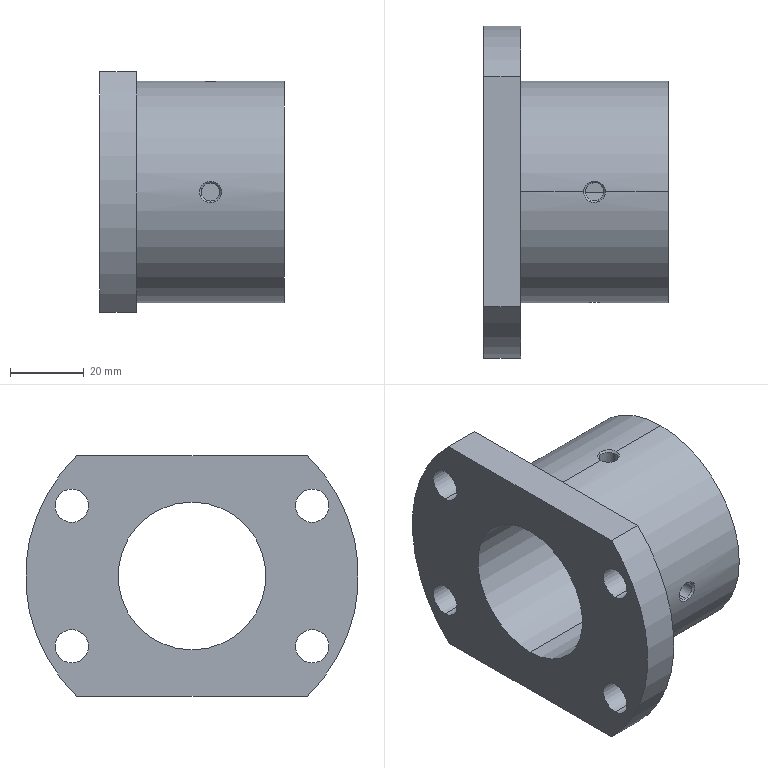Part | STEP file | sthc40 | 1 solid | 27 faces | box 50 x 90 x 65 mm | volume 100252 mm3 | cylinder 18 | plane 5 | cone 4 | commonest cylinder face diameters 9 x8 4.917 x4 40 x2 60 x2 90 x2